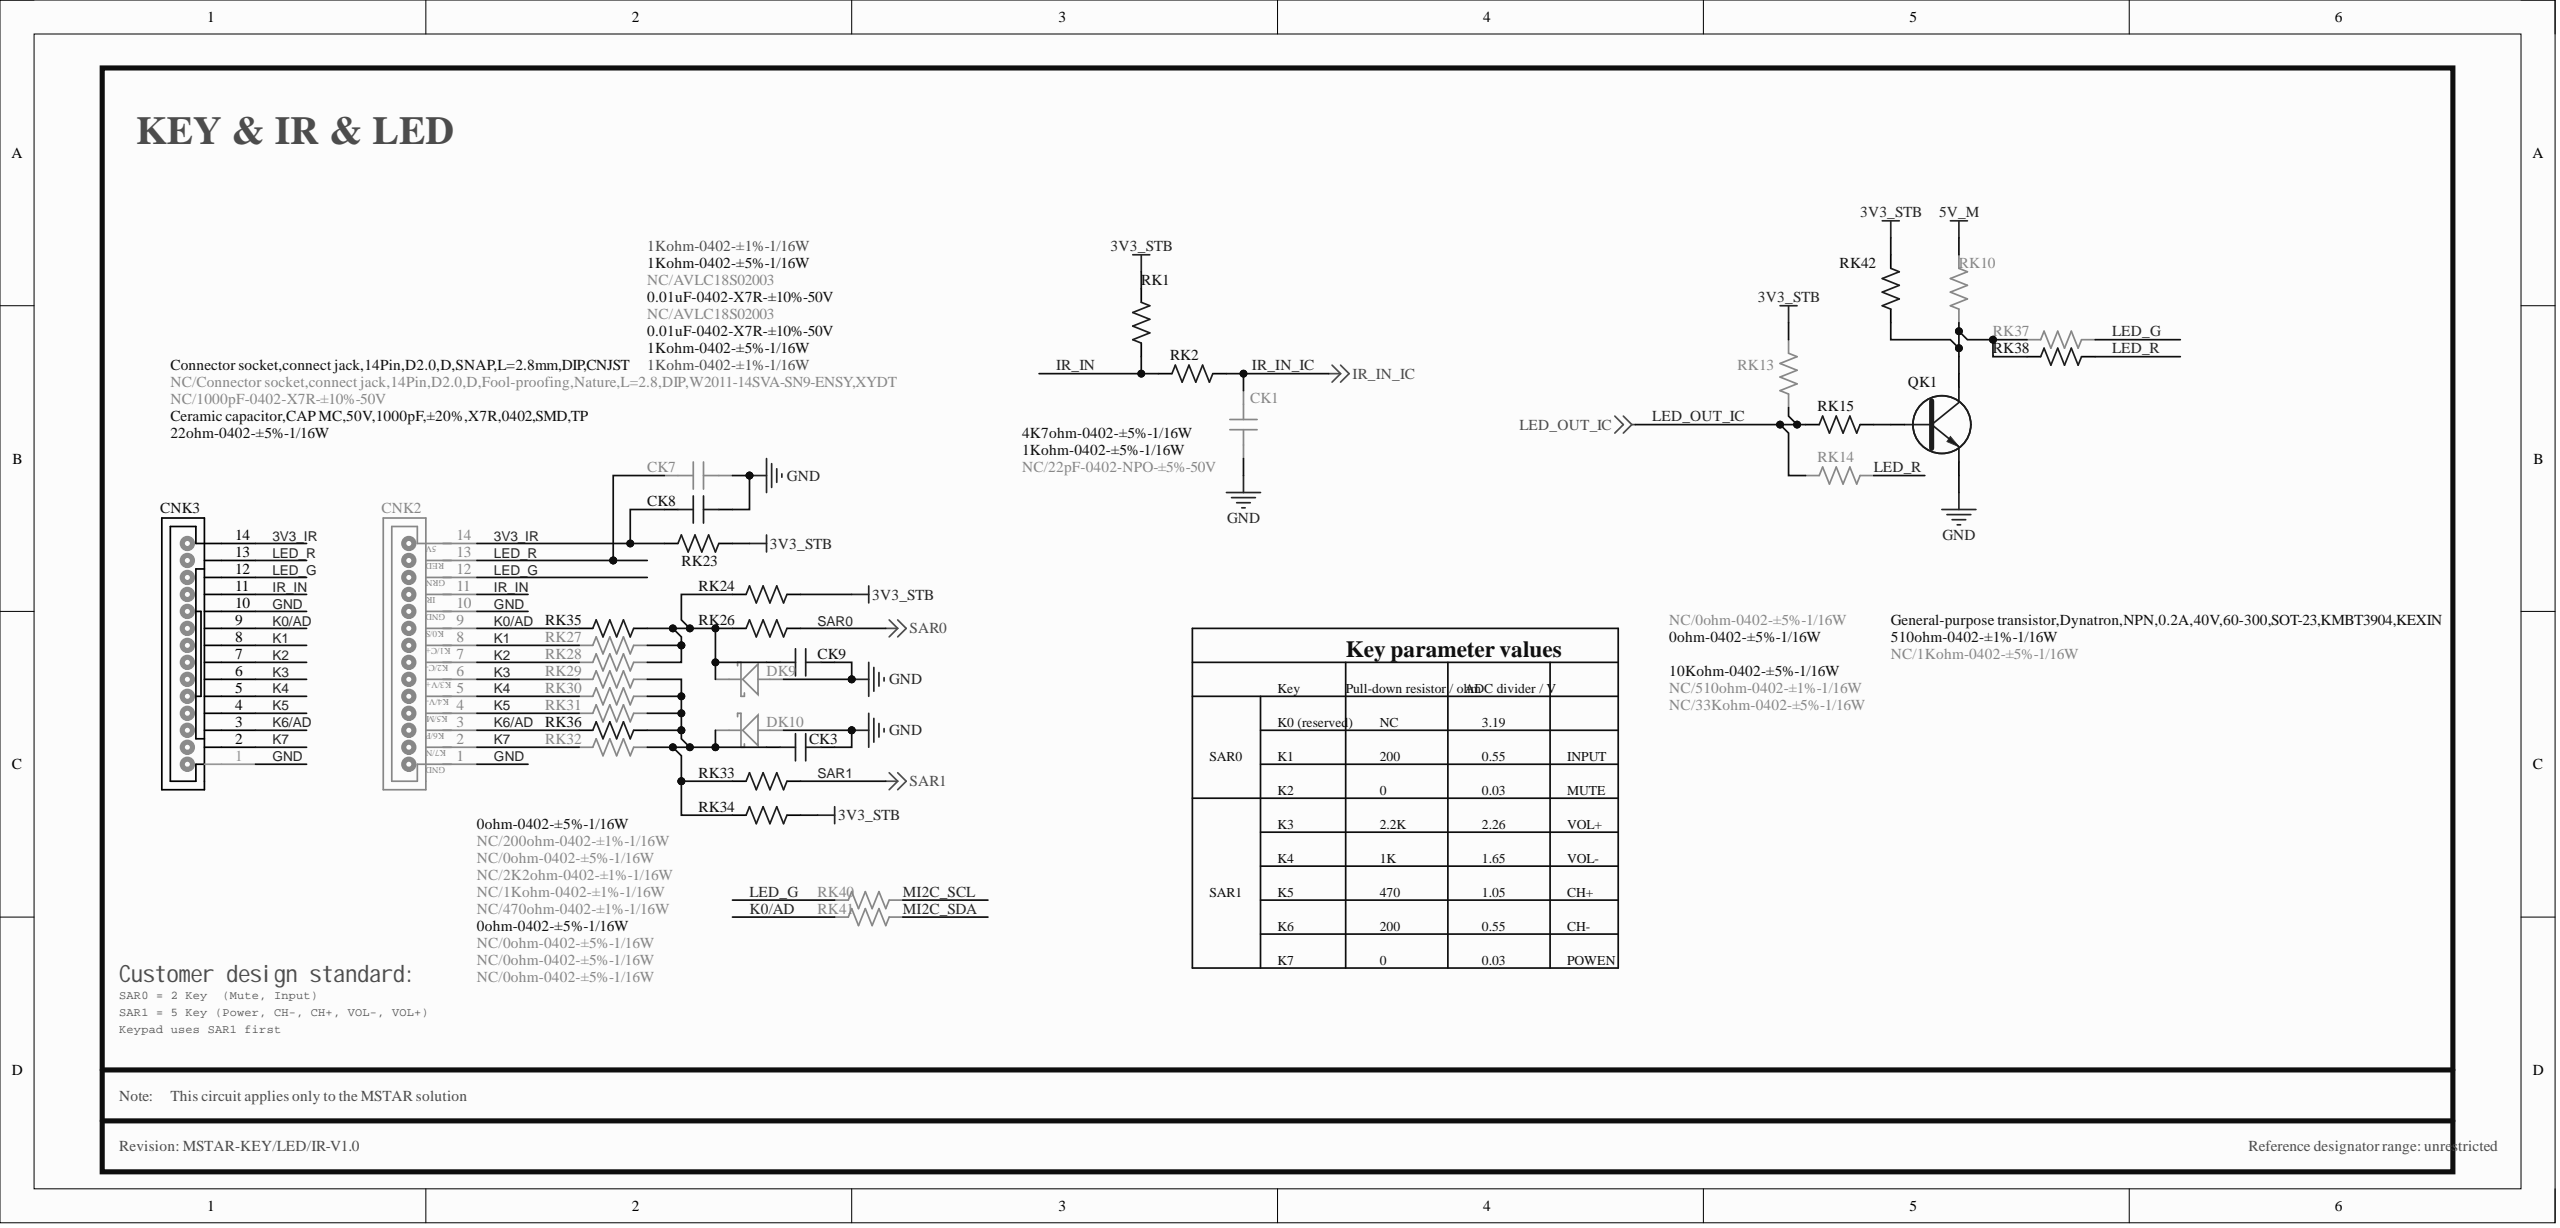Circuit board | Altium Designer | 1029 parts | 642 nets | one sheet of the schematic
Parts on this sheet (reference | value | footprint):
CK1 | NC/22pF-0402-NPO-±5%-50V | C0402
CK3 | 0.01uF-0402-X7R-±10%-50V | C0402
CK7 | NC/1000pF-0402-X7R-±10%-50V | C0402
CK8 | Ceramic capacitor,CAP MC,50V,1000pF,±20%,X7R,0402,SMD,TP | C0402
CK9 | 0.01uF-0402-X7R-±10%-50V | C0402
CNK2 | NC/Connector socket,connect jack,14Pin,D2.0,D,Fool-proofing,Nature,L=2.8,DIP,W2011-14SVA-SN9-ENSY,XYDT | SIP14/2.0D-2
CNK3 | Connector socket,connect jack,14Pin,D2.0,D,SNAP,L=2.8mm,DIP,CNJST | SIP14/2.0D-5
DK9 | NC/AVLC18S02003 | DIODE-S0402
DK10 | NC/AVLC18S02003 | DIODE-S0402
QK1 | General-purpose transistor,Dynatron,NPN,0.2A,40V,60-300,SOT-23,KMBT3904,KEXIN | SOT-23
RK1 | 4K7ohm-0402-±5%-1/16W | R0402
RK2 | 1Kohm-0402-±5%-1/16W | R0402
RK10 | NC/1Kohm-0402-±5%-1/16W | R0402
RK13 | NC/33Kohm-0402-±5%-1/16W | R0402
RK14 | NC/510ohm-0402-±1%-1/16W | R0402
RK15 | 10Kohm-0402-±5%-1/16W | R0402
RK23 | 22ohm-0402-±5%-1/16W | R0402
RK24 | 1Kohm-0402-±1%-1/16W | R0402
RK26 | 1Kohm-0402-±5%-1/16W | R0402
RK27 | NC/200ohm-0402-±1%-1/16W | R0402
RK28 | NC/0ohm-0402-±5%-1/16W | R0402
RK29 | NC/2K2ohm-0402-±1%-1/16W | R0402
RK30 | NC/1Kohm-0402-±1%-1/16W | R0402
RK31 | NC/470ohm-0402-±1%-1/16W | R0402
RK32 | NC/0ohm-0402-±5%-1/16W | R0402
RK33 | 1Kohm-0402-±5%-1/16W | R0402
RK34 | 1Kohm-0402-±1%-1/16W | R0402
RK35 | 0ohm-0402-±5%-1/16W | R0402
RK36 | 0ohm-0402-±5%-1/16W | R0402
RK37 | NC/0ohm-0402-±5%-1/16W | R0402
RK38 | 0ohm-0402-±5%-1/16W | R0402
RK40 | NC/0ohm-0402-±5%-1/16W | R0402
RK41 | NC/0ohm-0402-±5%-1/16W | R0402
RK42 | 510ohm-0402-±1%-1/16W | R0402
Nets of these parts (net: part-pin ...):
SAR1: RK33-1
SAR0: RK26-1
NetQK1_C: QK1-C RK10-1 RK37-2 RK38-2 RK42-1
NetQK1_B: QK1-B RK15-1
NetCK9_2: CK9-2 DK9-K RK24-1 RK26-2 RK27-1 RK28-1 RK35-1
NetCK3_2: CK3-2 DK10-K RK29-1 RK30-2 RK31-1 RK32-1 RK33-2 RK34-1 RK36-1
MI2C_SDA: RK41-1
MI2C_SCL: RK40-1
LED_R: CK7-2 CNK2-13 CNK3-13 RK14-2 RK38-1
LED_OUT_IC: RK13-1 RK14-1 RK15-2
LED_G: CNK2-12 CNK3-12 RK37-1 RK40-2
K7: CNK2-2 CNK3-2 RK32-2
K6/AD: CNK2-3 CNK3-3 RK36-2
K5: CNK2-4 CNK3-4 RK31-2
K4: CNK2-5 CNK3-5 RK30-1
K3: CNK2-6 CNK3-6 RK29-2
K2: CNK2-7 CNK3-7 RK28-2
K1: CNK2-8 CNK3-8 RK27-2
K0/AD: CNK2-9 CNK3-9 RK35-2 RK41-2
IR_IN_IC: CK1-2 RK2-2
IR_IN: CNK2-11 CNK3-11 RK1-1 RK2-1
GND: CK1-1 CK3-1 CK7-1 CK8-1 CK9-1 CNK2-1 CNK2-10 CNK3-1 CNK3-10 DK9-A DK10-A QK1-E
5V_M: RK10-2
3V3_STB: RK1-2 RK13-2 RK23-1 RK24-2 RK34-2 RK42-2
3V3_IR: CK8-2 CNK2-14 CNK3-14 RK23-2